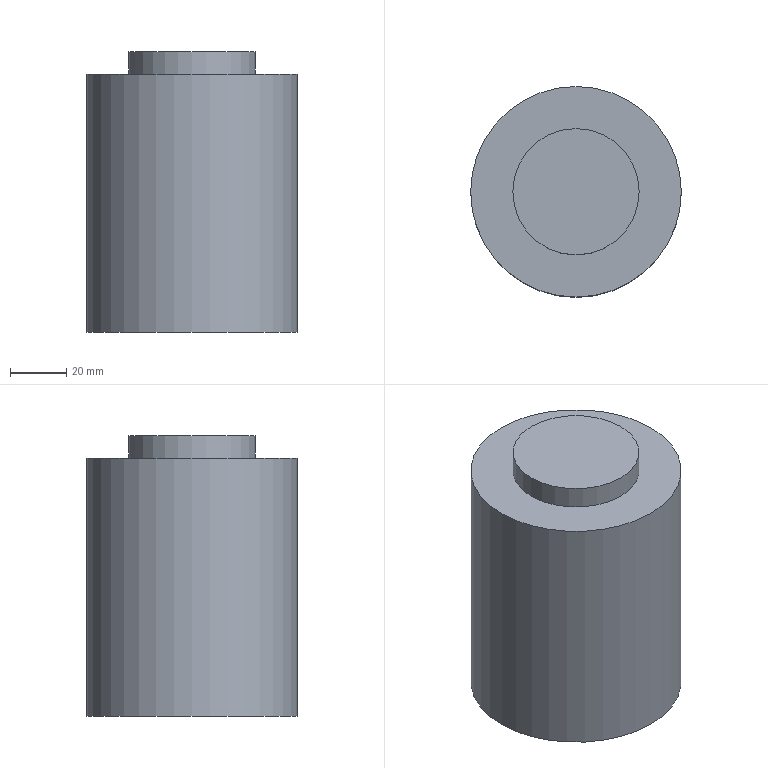Part | NX | features solid 2 | 1 solid | 5 faces | box 75 x 75 x 100 mm | volume 419167 mm3 | plane 3 | cylinder 2 | commonest cylinder face diameters 45 x1 75 x1
STEP:
#1=CARTESIAN_POINT('',(-1207.5,660.,-73.));
#2=VERTEX_POINT('',#1);
#3=CARTESIAN_POINT('',(-1185.,660.,-73.));
#4=DIRECTION('',(0.,0.,1.));
#5=DIRECTION('',(-1.,0.,0.));
#6=AXIS2_PLACEMENT_3D('',#3,#4,#5);
#7=CIRCLE('',#6,22.5);
#8=EDGE_CURVE('',#2,#2,#7,.T.);
#9=ORIENTED_EDGE('',*,*,#8,.F.);
#10=EDGE_LOOP('',(#9));
#11=FACE_BOUND('',#10,.T.);
#12=CARTESIAN_POINT('',(-1147.5,660.,-73.));
#13=VERTEX_POINT('',#12);
#14=CARTESIAN_POINT('',(-1185.,660.,-73.));
#15=DIRECTION('',(0.,0.,-1.));
#16=DIRECTION('',(1.,0.,0.));
#17=AXIS2_PLACEMENT_3D('',#14,#15,#16);
#18=CIRCLE('',#17,37.5);
#19=EDGE_CURVE('',#13,#13,#18,.T.);
#20=ORIENTED_EDGE('',*,*,#19,.F.);
#21=EDGE_LOOP('',(#20));
#22=FACE_BOUND('',#21,.T.);
#23=CARTESIAN_POINT('',(-1185.,660.,-73.));
#24=DIRECTION('',(0.,0.,1.));
#25=DIRECTION('',(-1.,0.,0.));
#26=AXIS2_PLACEMENT_3D('',#23,#24,#25);
#27=PLANE('',#26);
#28=ADVANCED_FACE('',(#11,#22),#27,.T.);
#29=CARTESIAN_POINT('',(-1147.5,660.,-165.));
#30=VERTEX_POINT('',#29);
#31=CARTESIAN_POINT('',(-1185.,660.,-165.));
#32=DIRECTION('',(0.,0.,-1.));
#33=DIRECTION('',(1.,0.,0.));
#34=AXIS2_PLACEMENT_3D('',#31,#32,#33);
#35=CIRCLE('',#34,37.5);
#36=EDGE_CURVE('',#30,#30,#35,.F.);
#37=ORIENTED_EDGE('',*,*,#36,.F.);
#38=EDGE_LOOP('',(#37));
#39=FACE_BOUND('',#38,.T.);
#40=CARTESIAN_POINT('',(-1225.,723.5,-165.));
#41=DIRECTION('',(0.,0.,-1.));
#42=DIRECTION('',(1.,0.,0.));
#43=AXIS2_PLACEMENT_3D('',#40,#41,#42);
#44=PLANE('',#43);
#45=ADVANCED_FACE('',(#39),#44,.T.);
#46=ORIENTED_EDGE('',*,*,#19,.T.);
#47=EDGE_LOOP('',(#46));
#48=FACE_BOUND('',#47,.T.);
#49=ORIENTED_EDGE('',*,*,#36,.T.);
#50=EDGE_LOOP('',(#49));
#51=FACE_BOUND('',#50,.T.);
#52=CARTESIAN_POINT('',(-1185.,660.,-74.));
#53=DIRECTION('',(0.,0.,1.));
#54=DIRECTION('',(-1.,0.,0.));
#55=AXIS2_PLACEMENT_3D('',#52,#53,#54);
#56=CYLINDRICAL_SURFACE('',#55,37.5);
#57=ADVANCED_FACE('',(#48,#51),#56,.T.);
#58=CARTESIAN_POINT('',(-1207.5,660.,-65.));
#59=VERTEX_POINT('',#58);
#60=CARTESIAN_POINT('',(-1185.,660.,-65.));
#61=DIRECTION('',(0.,0.,1.));
#62=DIRECTION('',(-1.,0.,0.));
#63=AXIS2_PLACEMENT_3D('',#60,#61,#62);
#64=CIRCLE('',#63,22.5);
#65=EDGE_CURVE('',#59,#59,#64,.T.);
#66=ORIENTED_EDGE('',*,*,#65,.T.);
#67=EDGE_LOOP('',(#66));
#68=FACE_BOUND('',#67,.T.);
#69=CARTESIAN_POINT('',(-1185.,660.,-65.));
#70=DIRECTION('',(0.,0.,1.));
#71=DIRECTION('',(-1.,0.,0.));
#72=AXIS2_PLACEMENT_3D('',#69,#70,#71);
#73=PLANE('',#72);
#74=ADVANCED_FACE('',(#68),#73,.T.);
#75=ORIENTED_EDGE('',*,*,#65,.F.);
#76=EDGE_LOOP('',(#75));
#77=FACE_BOUND('',#76,.T.);
#78=ORIENTED_EDGE('',*,*,#8,.T.);
#79=EDGE_LOOP('',(#78));
#80=FACE_BOUND('',#79,.T.);
#81=CARTESIAN_POINT('',(-1185.,660.,-73.));
#82=DIRECTION('',(0.,0.,1.));
#83=DIRECTION('',(-1.,0.,0.));
#84=AXIS2_PLACEMENT_3D('',#81,#82,#83);
#85=CYLINDRICAL_SURFACE('',#84,22.5);
#86=ADVANCED_FACE('',(#77,#80),#85,.T.);
#87=CLOSED_SHELL('',(#28,#45,#57,#74,#86));
#88=MANIFOLD_SOLID_BREP('',#87);
#89=(LENGTH_UNIT()NAMED_UNIT(*)SI_UNIT(.MILLI.,.METRE.));
#90=UNCERTAINTY_MEASURE_WITH_UNIT(LENGTH_MEASURE(0.00001),#89,'','');
#91=(NAMED_UNIT(*)PLANE_ANGLE_UNIT()SI_UNIT($,.RADIAN.));
#92=(NAMED_UNIT(*)SI_UNIT($,.STERADIAN.)SOLID_ANGLE_UNIT());
#93=(GEOMETRIC_REPRESENTATION_CONTEXT(3)GLOBAL_UNCERTAINTY_ASSIGNED_CONTEXT((#90))GLOBAL_UNIT_ASSIGNED_CONTEXT((#89,#91,#92))REPRESENTATION_CONTEXT('',''));
#94=ADVANCED_BREP_SHAPE_REPRESENTATION('',(#88),#93);